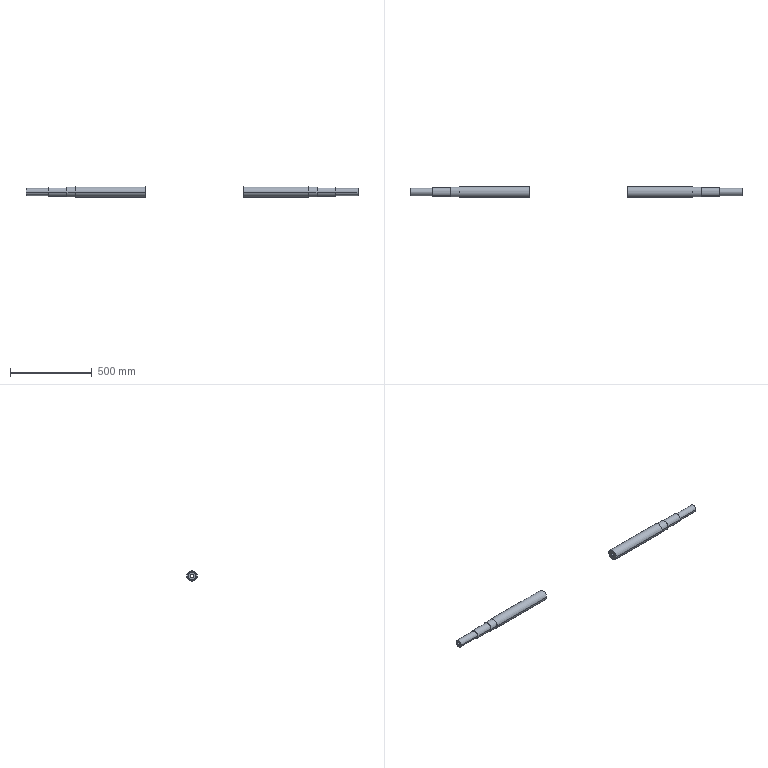Part | STEP file | Axle | 2 solids | 30 faces | box 2025 x 64 x 64 mm | volume 3440421 mm3 | cylinder 20 | plane 10 | commonest cylinder face diameters 20 x4 45 x4 54 x4 60 x4 64 x4
STEP:
#1=CARTESIAN_POINT('',(-712.5,-30.,0.));
#2=VERTEX_POINT('',#1);
#3=CARTESIAN_POINT('',(-712.5,30.,0.));
#4=VERTEX_POINT('',#3);
#5=CARTESIAN_POINT('',(-712.5,0.,0.));
#6=DIRECTION('',(-1.,0.,0.));
#7=DIRECTION('',(0.,-1.,0.));
#8=AXIS2_PLACEMENT_3D('',#5,#6,#7);
#9=CIRCLE('',#8,30.);
#10=EDGE_CURVE('',#2,#4,#9,.T.);
#11=ORIENTED_EDGE('',*,*,#10,.T.);
#12=CARTESIAN_POINT('',(-762.5,30.,0.));
#13=VERTEX_POINT('',#12);
#14=CARTESIAN_POINT('',(-1012.5,30.,0.));
#15=DIRECTION('',(-1.,0.,0.));
#16=VECTOR('',#15,1000.);
#17=LINE('',#14,#16);
#18=EDGE_CURVE('',#4,#13,#17,.T.);
#19=ORIENTED_EDGE('',*,*,#18,.T.);
#20=CARTESIAN_POINT('',(-762.5,-30.,0.));
#21=VERTEX_POINT('',#20);
#22=CARTESIAN_POINT('',(-762.5,0.,0.));
#23=DIRECTION('',(-1.,0.,0.));
#24=DIRECTION('',(0.,-1.,0.));
#25=AXIS2_PLACEMENT_3D('',#22,#23,#24);
#26=CIRCLE('',#25,30.);
#27=EDGE_CURVE('',#21,#13,#26,.T.);
#28=ORIENTED_EDGE('',*,*,#27,.F.);
#29=CARTESIAN_POINT('',(-1012.5,-30.,0.));
#30=DIRECTION('',(-1.,0.,0.));
#31=VECTOR('',#30,1000.);
#32=LINE('',#29,#31);
#33=EDGE_CURVE('',#2,#21,#32,.T.);
#34=ORIENTED_EDGE('',*,*,#33,.F.);
#35=EDGE_LOOP('',(#11,#19,#28,#34));
#36=FACE_OUTER_BOUND('',#35,.T.);
#37=CARTESIAN_POINT('',(-1012.5,0.,0.));
#38=DIRECTION('',(-1.,0.,0.));
#39=DIRECTION('',(0.,-1.,0.));
#40=AXIS2_PLACEMENT_3D('',#37,#38,#39);
#41=CYLINDRICAL_SURFACE('',#40,30.);
#42=ADVANCED_FACE('',(#36),#41,.T.);
#43=CARTESIAN_POINT('',(-762.5,-27.,0.));
#44=VERTEX_POINT('',#43);
#45=CARTESIAN_POINT('',(-762.5,27.,0.));
#46=VERTEX_POINT('',#45);
#47=CARTESIAN_POINT('',(-762.5,0.,0.));
#48=DIRECTION('',(-1.,0.,0.));
#49=DIRECTION('',(0.,-1.,0.));
#50=AXIS2_PLACEMENT_3D('',#47,#48,#49);
#51=CIRCLE('',#50,27.);
#52=EDGE_CURVE('',#44,#46,#51,.T.);
#53=ORIENTED_EDGE('',*,*,#52,.T.);
#54=CARTESIAN_POINT('',(-872.5,27.,0.));
#55=VERTEX_POINT('',#54);
#56=CARTESIAN_POINT('',(-1012.5,27.,0.));
#57=DIRECTION('',(-1.,0.,0.));
#58=VECTOR('',#57,1000.);
#59=LINE('',#56,#58);
#60=EDGE_CURVE('',#46,#55,#59,.T.);
#61=ORIENTED_EDGE('',*,*,#60,.T.);
#62=CARTESIAN_POINT('',(-872.5,-27.,0.));
#63=VERTEX_POINT('',#62);
#64=CARTESIAN_POINT('',(-872.5,0.,0.));
#65=DIRECTION('',(-1.,0.,0.));
#66=DIRECTION('',(0.,-1.,0.));
#67=AXIS2_PLACEMENT_3D('',#64,#65,#66);
#68=CIRCLE('',#67,27.);
#69=EDGE_CURVE('',#63,#55,#68,.T.);
#70=ORIENTED_EDGE('',*,*,#69,.F.);
#71=CARTESIAN_POINT('',(-1012.5,-27.,0.));
#72=DIRECTION('',(-1.,0.,0.));
#73=VECTOR('',#72,1000.);
#74=LINE('',#71,#73);
#75=EDGE_CURVE('',#44,#63,#74,.T.);
#76=ORIENTED_EDGE('',*,*,#75,.F.);
#77=EDGE_LOOP('',(#53,#61,#70,#76));
#78=FACE_OUTER_BOUND('',#77,.T.);
#79=CARTESIAN_POINT('',(-1012.5,0.,0.));
#80=DIRECTION('',(-1.,0.,0.));
#81=DIRECTION('',(0.,-1.,0.));
#82=AXIS2_PLACEMENT_3D('',#79,#80,#81);
#83=CYLINDRICAL_SURFACE('',#82,27.);
#84=ADVANCED_FACE('',(#78),#83,.T.);
#85=CARTESIAN_POINT('',(-872.5,-22.5,0.));
#86=VERTEX_POINT('',#85);
#87=CARTESIAN_POINT('',(-872.5,22.5,0.));
#88=VERTEX_POINT('',#87);
#89=CARTESIAN_POINT('',(-872.5,0.,0.));
#90=DIRECTION('',(-1.,0.,0.));
#91=DIRECTION('',(0.,-1.,0.));
#92=AXIS2_PLACEMENT_3D('',#89,#90,#91);
#93=CIRCLE('',#92,22.5);
#94=EDGE_CURVE('',#86,#88,#93,.T.);
#95=ORIENTED_EDGE('',*,*,#94,.T.);
#96=CARTESIAN_POINT('',(-1012.5,22.5,0.));
#97=VERTEX_POINT('',#96);
#98=CARTESIAN_POINT('',(-1012.5,22.5,0.));
#99=DIRECTION('',(-1.,0.,0.));
#100=VECTOR('',#99,1000.);
#101=LINE('',#98,#100);
#102=EDGE_CURVE('',#88,#97,#101,.T.);
#103=ORIENTED_EDGE('',*,*,#102,.T.);
#104=CARTESIAN_POINT('',(-1012.5,-22.5,0.));
#105=VERTEX_POINT('',#104);
#106=CARTESIAN_POINT('',(-1012.5,0.,0.));
#107=DIRECTION('',(-1.,0.,0.));
#108=DIRECTION('',(0.,-1.,0.));
#109=AXIS2_PLACEMENT_3D('',#106,#107,#108);
#110=CIRCLE('',#109,22.5);
#111=EDGE_CURVE('',#105,#97,#110,.T.);
#112=ORIENTED_EDGE('',*,*,#111,.F.);
#113=CARTESIAN_POINT('',(-1012.5,-22.5,0.));
#114=DIRECTION('',(-1.,0.,0.));
#115=VECTOR('',#114,1000.);
#116=LINE('',#113,#115);
#117=EDGE_CURVE('',#86,#105,#116,.T.);
#118=ORIENTED_EDGE('',*,*,#117,.F.);
#119=EDGE_LOOP('',(#95,#103,#112,#118));
#120=FACE_OUTER_BOUND('',#119,.T.);
#121=CARTESIAN_POINT('',(-1012.5,0.,0.));
#122=DIRECTION('',(-1.,0.,0.));
#123=DIRECTION('',(0.,-1.,0.));
#124=AXIS2_PLACEMENT_3D('',#121,#122,#123);
#125=CYLINDRICAL_SURFACE('',#124,22.5);
#126=ADVANCED_FACE('',(#120),#125,.T.);
#127=CARTESIAN_POINT('',(-284.662,-10.,0.));
#128=VERTEX_POINT('',#127);
#129=CARTESIAN_POINT('',(-284.662,10.,0.));
#130=VERTEX_POINT('',#129);
#131=CARTESIAN_POINT('',(-284.662,0.,0.));
#132=DIRECTION('',(1.,0.,0.));
#133=DIRECTION('',(0.,0.,1.));
#134=AXIS2_PLACEMENT_3D('',#131,#132,#133);
#135=CIRCLE('',#134,10.);
#136=EDGE_CURVE('',#128,#130,#135,.T.);
#137=ORIENTED_EDGE('',*,*,#136,.T.);
#138=CARTESIAN_POINT('',(-1012.5,10.,0.));
#139=VERTEX_POINT('',#138);
#140=CARTESIAN_POINT('',(1012.501,10.,0.));
#141=DIRECTION('',(-1.,0.,0.));
#142=VECTOR('',#141,1000.);
#143=LINE('',#140,#142);
#144=EDGE_CURVE('',#130,#139,#143,.T.);
#145=ORIENTED_EDGE('',*,*,#144,.T.);
#146=CARTESIAN_POINT('',(-1012.5,-10.,0.));
#147=VERTEX_POINT('',#146);
#148=CARTESIAN_POINT('',(-1012.5,0.,0.));
#149=DIRECTION('',(-1.,0.,0.));
#150=DIRECTION('',(0.,-1.,0.));
#151=AXIS2_PLACEMENT_3D('',#148,#149,#150);
#152=CIRCLE('',#151,10.);
#153=EDGE_CURVE('',#139,#147,#152,.T.);
#154=ORIENTED_EDGE('',*,*,#153,.T.);
#155=CARTESIAN_POINT('',(1012.501,-10.,0.));
#156=DIRECTION('',(-1.,0.,0.));
#157=VECTOR('',#156,1000.);
#158=LINE('',#155,#157);
#159=EDGE_CURVE('',#128,#147,#158,.T.);
#160=ORIENTED_EDGE('',*,*,#159,.F.);
#161=EDGE_LOOP('',(#137,#145,#154,#160));
#162=FACE_OUTER_BOUND('',#161,.T.);
#163=CARTESIAN_POINT('',(1012.501,0.,0.));
#164=DIRECTION('',(-1.,0.,0.));
#165=DIRECTION('',(0.,-1.,0.));
#166=AXIS2_PLACEMENT_3D('',#163,#164,#165);
#167=CYLINDRICAL_SURFACE('',#166,10.);
#168=ADVANCED_FACE('',(#162),#167,.F.);
#169=CARTESIAN_POINT('',(-284.662,-32.,0.));
#170=VERTEX_POINT('',#169);
#171=CARTESIAN_POINT('',(-284.662,32.,0.));
#172=VERTEX_POINT('',#171);
#173=CARTESIAN_POINT('',(-284.662,0.,0.));
#174=DIRECTION('',(-1.,0.,0.));
#175=DIRECTION('',(0.,0.,1.));
#176=AXIS2_PLACEMENT_3D('',#173,#174,#175);
#177=CIRCLE('',#176,32.);
#178=EDGE_CURVE('',#170,#172,#177,.T.);
#179=ORIENTED_EDGE('',*,*,#178,.T.);
#180=CARTESIAN_POINT('',(-712.5,32.,0.));
#181=VERTEX_POINT('',#180);
#182=CARTESIAN_POINT('',(-1012.5,32.,0.));
#183=DIRECTION('',(-1.,0.,0.));
#184=VECTOR('',#183,1000.);
#185=LINE('',#182,#184);
#186=EDGE_CURVE('',#172,#181,#185,.T.);
#187=ORIENTED_EDGE('',*,*,#186,.T.);
#188=CARTESIAN_POINT('',(-712.5,-32.,0.));
#189=VERTEX_POINT('',#188);
#190=CARTESIAN_POINT('',(-712.5,0.,0.));
#191=DIRECTION('',(-1.,0.,0.));
#192=DIRECTION('',(0.,-1.,0.));
#193=AXIS2_PLACEMENT_3D('',#190,#191,#192);
#194=CIRCLE('',#193,32.);
#195=EDGE_CURVE('',#189,#181,#194,.T.);
#196=ORIENTED_EDGE('',*,*,#195,.F.);
#197=CARTESIAN_POINT('',(-1012.5,-32.,0.));
#198=DIRECTION('',(-1.,0.,0.));
#199=VECTOR('',#198,1000.);
#200=LINE('',#197,#199);
#201=EDGE_CURVE('',#170,#189,#200,.T.);
#202=ORIENTED_EDGE('',*,*,#201,.F.);
#203=EDGE_LOOP('',(#179,#187,#196,#202));
#204=FACE_OUTER_BOUND('',#203,.T.);
#205=CARTESIAN_POINT('',(-1012.5,0.,0.));
#206=DIRECTION('',(-1.,0.,0.));
#207=DIRECTION('',(0.,-1.,0.));
#208=AXIS2_PLACEMENT_3D('',#205,#206,#207);
#209=CYLINDRICAL_SURFACE('',#208,32.);
#210=ADVANCED_FACE('',(#204),#209,.T.);
#211=ORIENTED_EDGE('',*,*,#186,.F.);
#212=CARTESIAN_POINT('',(-284.662,0.,0.));
#213=DIRECTION('',(-1.,0.,0.));
#214=DIRECTION('',(0.,0.,1.));
#215=AXIS2_PLACEMENT_3D('',#212,#213,#214);
#216=CIRCLE('',#215,32.);
#217=EDGE_CURVE('',#172,#170,#216,.T.);
#218=ORIENTED_EDGE('',*,*,#217,.T.);
#219=ORIENTED_EDGE('',*,*,#201,.T.);
#220=CARTESIAN_POINT('',(-712.5,0.,0.));
#221=DIRECTION('',(-1.,0.,0.));
#222=DIRECTION('',(0.,-1.,0.));
#223=AXIS2_PLACEMENT_3D('',#220,#221,#222);
#224=CIRCLE('',#223,32.);
#225=EDGE_CURVE('',#181,#189,#224,.T.);
#226=ORIENTED_EDGE('',*,*,#225,.F.);
#227=EDGE_LOOP('',(#211,#218,#219,#226));
#228=FACE_OUTER_BOUND('',#227,.T.);
#229=CARTESIAN_POINT('',(-1012.5,0.,0.));
#230=DIRECTION('',(-1.,0.,0.));
#231=DIRECTION('',(0.,-1.,0.));
#232=AXIS2_PLACEMENT_3D('',#229,#230,#231);
#233=CYLINDRICAL_SURFACE('',#232,32.);
#234=ADVANCED_FACE('',(#228),#233,.T.);
#235=ORIENTED_EDGE('',*,*,#144,.F.);
#236=CARTESIAN_POINT('',(-284.662,0.,0.));
#237=DIRECTION('',(1.,0.,0.));
#238=DIRECTION('',(0.,0.,1.));
#239=AXIS2_PLACEMENT_3D('',#236,#237,#238);
#240=CIRCLE('',#239,10.);
#241=EDGE_CURVE('',#130,#128,#240,.T.);
#242=ORIENTED_EDGE('',*,*,#241,.T.);
#243=ORIENTED_EDGE('',*,*,#159,.T.);
#244=CARTESIAN_POINT('',(-1012.5,0.,0.));
#245=DIRECTION('',(-1.,0.,0.));
#246=DIRECTION('',(0.,-1.,0.));
#247=AXIS2_PLACEMENT_3D('',#244,#245,#246);
#248=CIRCLE('',#247,10.);
#249=EDGE_CURVE('',#147,#139,#248,.T.);
#250=ORIENTED_EDGE('',*,*,#249,.T.);
#251=EDGE_LOOP('',(#235,#242,#243,#250));
#252=FACE_OUTER_BOUND('',#251,.T.);
#253=CARTESIAN_POINT('',(1012.501,0.,0.));
#254=DIRECTION('',(-1.,0.,0.));
#255=DIRECTION('',(0.,-1.,0.));
#256=AXIS2_PLACEMENT_3D('',#253,#254,#255);
#257=CYLINDRICAL_SURFACE('',#256,10.);
#258=ADVANCED_FACE('',(#252),#257,.F.);
#259=ORIENTED_EDGE('',*,*,#249,.F.);
#260=ORIENTED_EDGE('',*,*,#153,.F.);
#261=EDGE_LOOP('',(#259,#260));
#262=FACE_BOUND('',#261,.T.);
#263=ORIENTED_EDGE('',*,*,#111,.T.);
#264=CARTESIAN_POINT('',(-1012.5,0.,0.));
#265=DIRECTION('',(-1.,0.,0.));
#266=DIRECTION('',(0.,-1.,0.));
#267=AXIS2_PLACEMENT_3D('',#264,#265,#266);
#268=CIRCLE('',#267,22.5);
#269=EDGE_CURVE('',#97,#105,#268,.T.);
#270=ORIENTED_EDGE('',*,*,#269,.T.);
#271=EDGE_LOOP('',(#263,#270));
#272=FACE_OUTER_BOUND('',#271,.T.);
#273=CARTESIAN_POINT('',(-1012.5,0.,0.));
#274=DIRECTION('',(1.,0.,0.));
#275=DIRECTION('',(0.,1.,0.));
#276=AXIS2_PLACEMENT_3D('',#273,#274,#275);
#277=PLANE('',#276);
#278=ADVANCED_FACE('',(#262,#272),#277,.F.);
#279=ORIENTED_EDGE('',*,*,#102,.F.);
#280=CARTESIAN_POINT('',(-872.5,0.,0.));
#281=DIRECTION('',(-1.,0.,0.));
#282=DIRECTION('',(0.,-1.,0.));
#283=AXIS2_PLACEMENT_3D('',#280,#281,#282);
#284=CIRCLE('',#283,22.5);
#285=EDGE_CURVE('',#88,#86,#284,.T.);
#286=ORIENTED_EDGE('',*,*,#285,.T.);
#287=ORIENTED_EDGE('',*,*,#117,.T.);
#288=ORIENTED_EDGE('',*,*,#269,.F.);
#289=EDGE_LOOP('',(#279,#286,#287,#288));
#290=FACE_OUTER_BOUND('',#289,.T.);
#291=CARTESIAN_POINT('',(-1012.5,0.,0.));
#292=DIRECTION('',(-1.,0.,0.));
#293=DIRECTION('',(0.,-1.,0.));
#294=AXIS2_PLACEMENT_3D('',#291,#292,#293);
#295=CYLINDRICAL_SURFACE('',#294,22.5);
#296=ADVANCED_FACE('',(#290),#295,.T.);
#297=ORIENTED_EDGE('',*,*,#94,.F.);
#298=ORIENTED_EDGE('',*,*,#285,.F.);
#299=EDGE_LOOP('',(#297,#298));
#300=FACE_BOUND('',#299,.T.);
#301=ORIENTED_EDGE('',*,*,#69,.T.);
#302=CARTESIAN_POINT('',(-872.5,0.,0.));
#303=DIRECTION('',(-1.,0.,0.));
#304=DIRECTION('',(0.,-1.,0.));
#305=AXIS2_PLACEMENT_3D('',#302,#303,#304);
#306=CIRCLE('',#305,27.);
#307=EDGE_CURVE('',#55,#63,#306,.T.);
#308=ORIENTED_EDGE('',*,*,#307,.T.);
#309=EDGE_LOOP('',(#301,#308));
#310=FACE_OUTER_BOUND('',#309,.T.);
#311=CARTESIAN_POINT('',(-872.5,22.5,0.));
#312=DIRECTION('',(1.,0.,0.));
#313=DIRECTION('',(0.,1.,0.));
#314=AXIS2_PLACEMENT_3D('',#311,#312,#313);
#315=PLANE('',#314);
#316=ADVANCED_FACE('',(#300,#310),#315,.F.);
#317=ORIENTED_EDGE('',*,*,#60,.F.);
#318=CARTESIAN_POINT('',(-762.5,0.,0.));
#319=DIRECTION('',(-1.,0.,0.));
#320=DIRECTION('',(0.,-1.,0.));
#321=AXIS2_PLACEMENT_3D('',#318,#319,#320);
#322=CIRCLE('',#321,27.);
#323=EDGE_CURVE('',#46,#44,#322,.T.);
#324=ORIENTED_EDGE('',*,*,#323,.T.);
#325=ORIENTED_EDGE('',*,*,#75,.T.);
#326=ORIENTED_EDGE('',*,*,#307,.F.);
#327=EDGE_LOOP('',(#317,#324,#325,#326));
#328=FACE_OUTER_BOUND('',#327,.T.);
#329=CARTESIAN_POINT('',(-1012.5,0.,0.));
#330=DIRECTION('',(-1.,0.,0.));
#331=DIRECTION('',(0.,-1.,0.));
#332=AXIS2_PLACEMENT_3D('',#329,#330,#331);
#333=CYLINDRICAL_SURFACE('',#332,27.);
#334=ADVANCED_FACE('',(#328),#333,.T.);
#335=ORIENTED_EDGE('',*,*,#52,.F.);
#336=ORIENTED_EDGE('',*,*,#323,.F.);
#337=EDGE_LOOP('',(#335,#336));
#338=FACE_BOUND('',#337,.T.);
#339=ORIENTED_EDGE('',*,*,#27,.T.);
#340=CARTESIAN_POINT('',(-762.5,0.,0.));
#341=DIRECTION('',(-1.,0.,0.));
#342=DIRECTION('',(0.,-1.,0.));
#343=AXIS2_PLACEMENT_3D('',#340,#341,#342);
#344=CIRCLE('',#343,30.);
#345=EDGE_CURVE('',#13,#21,#344,.T.);
#346=ORIENTED_EDGE('',*,*,#345,.T.);
#347=EDGE_LOOP('',(#339,#346));
#348=FACE_OUTER_BOUND('',#347,.T.);
#349=CARTESIAN_POINT('',(-762.5,30.,0.));
#350=DIRECTION('',(1.,0.,0.));
#351=DIRECTION('',(0.,1.,0.));
#352=AXIS2_PLACEMENT_3D('',#349,#350,#351);
#353=PLANE('',#352);
#354=ADVANCED_FACE('',(#338,#348),#353,.F.);
#355=ORIENTED_EDGE('',*,*,#18,.F.);
#356=CARTESIAN_POINT('',(-712.5,0.,0.));
#357=DIRECTION('',(-1.,0.,0.));
#358=DIRECTION('',(0.,-1.,0.));
#359=AXIS2_PLACEMENT_3D('',#356,#357,#358);
#360=CIRCLE('',#359,30.);
#361=EDGE_CURVE('',#4,#2,#360,.T.);
#362=ORIENTED_EDGE('',*,*,#361,.T.);
#363=ORIENTED_EDGE('',*,*,#33,.T.);
#364=ORIENTED_EDGE('',*,*,#345,.F.);
#365=EDGE_LOOP('',(#355,#362,#363,#364));
#366=FACE_OUTER_BOUND('',#365,.T.);
#367=CARTESIAN_POINT('',(-1012.5,0.,0.));
#368=DIRECTION('',(-1.,0.,0.));
#369=DIRECTION('',(0.,-1.,0.));
#370=AXIS2_PLACEMENT_3D('',#367,#368,#369);
#371=CYLINDRICAL_SURFACE('',#370,30.);
#372=ADVANCED_FACE('',(#366),#371,.T.);
#373=ORIENTED_EDGE('',*,*,#10,.F.);
#374=ORIENTED_EDGE('',*,*,#361,.F.);
#375=EDGE_LOOP('',(#373,#374));
#376=FACE_BOUND('',#375,.T.);
#377=ORIENTED_EDGE('',*,*,#195,.T.);
#378=ORIENTED_EDGE('',*,*,#225,.T.);
#379=EDGE_LOOP('',(#377,#378));
#380=FACE_OUTER_BOUND('',#379,.T.);
#381=CARTESIAN_POINT('',(-712.5,30.,0.));
#382=DIRECTION('',(1.,0.,0.));
#383=DIRECTION('',(0.,1.,0.));
#384=AXIS2_PLACEMENT_3D('',#381,#382,#383);
#385=PLANE('',#384);
#386=ADVANCED_FACE('',(#376,#380),#385,.F.);
#387=ORIENTED_EDGE('',*,*,#136,.F.);
#388=ORIENTED_EDGE('',*,*,#241,.F.);
#389=EDGE_LOOP('',(#387,#388));
#390=FACE_BOUND('',#389,.T.);
#391=ORIENTED_EDGE('',*,*,#178,.F.);
#392=ORIENTED_EDGE('',*,*,#217,.F.);
#393=EDGE_LOOP('',(#391,#392));
#394=FACE_OUTER_BOUND('',#393,.T.);
#395=CARTESIAN_POINT('',(-284.662,-103.,59.586));
#396=DIRECTION('',(-1.,0.,0.));
#397=DIRECTION('',(0.,0.,1.));
#398=AXIS2_PLACEMENT_3D('',#395,#396,#397);
#399=PLANE('',#398);
#400=ADVANCED_FACE('',(#390,#394),#399,.F.);
#401=CLOSED_SHELL('',(#42,#84,#126,#168,#210,#234,#258,#278,#296,#316,#334,#354,#372,#386,#400));
#402=MANIFOLD_SOLID_BREP('',#401);
#403=CARTESIAN_POINT('',(1012.5,-10.,0.));
#404=VERTEX_POINT('',#403);
#405=CARTESIAN_POINT('',(1012.5,10.,0.));
#406=VERTEX_POINT('',#405);
#407=CARTESIAN_POINT('',(1012.5,0.,0.));
#408=DIRECTION('',(1.,0.,0.));
#409=DIRECTION('',(0.,-1.,0.));
#410=AXIS2_PLACEMENT_3D('',#407,#408,#409);
#411=CIRCLE('',#410,10.);
#412=EDGE_CURVE('',#404,#406,#411,.T.);
#413=ORIENTED_EDGE('',*,*,#412,.T.);
#414=CARTESIAN_POINT('',(314.592,10.,0.));
#415=VERTEX_POINT('',#414);
#416=CARTESIAN_POINT('',(1012.501,10.,0.));
#417=DIRECTION('',(-1.,0.,0.));
#418=VECTOR('',#417,1000.);
#419=LINE('',#416,#418);
#420=EDGE_CURVE('',#406,#415,#419,.T.);
#421=ORIENTED_EDGE('',*,*,#420,.T.);
#422=CARTESIAN_POINT('',(314.592,-10.,0.));
#423=VERTEX_POINT('',#422);
#424=CARTESIAN_POINT('',(314.592,0.,0.));
#425=DIRECTION('',(-1.,0.,0.));
#426=DIRECTION('',(0.,0.,-1.));
#427=AXIS2_PLACEMENT_3D('',#424,#425,#426);
#428=CIRCLE('',#427,10.);
#429=EDGE_CURVE('',#415,#423,#428,.T.);
#430=ORIENTED_EDGE('',*,*,#429,.T.);
#431=CARTESIAN_POINT('',(1012.501,-10.,0.));
#432=DIRECTION('',(-1.,0.,0.));
#433=VECTOR('',#432,1000.);
#434=LINE('',#431,#433);
#435=EDGE_CURVE('',#404,#423,#434,.T.);
#436=ORIENTED_EDGE('',*,*,#435,.F.);
#437=EDGE_LOOP('',(#413,#421,#430,#436));
#438=FACE_OUTER_BOUND('',#437,.T.);
#439=CARTESIAN_POINT('',(1012.501,0.,0.));
#440=DIRECTION('',(-1.,0.,0.));
#441=DIRECTION('',(0.,-1.,0.));
#442=AXIS2_PLACEMENT_3D('',#439,#440,#441);
#443=CYLINDRICAL_SURFACE('',#442,10.);
#444=ADVANCED_FACE('',(#438),#443,.F.);
#445=CARTESIAN_POINT('',(1012.5,-22.5,0.));
#446=VERTEX_POINT('',#445);
#447=CARTESIAN_POINT('',(1012.5,22.5,0.));
#448=VERTEX_POINT('',#447);
#449=CARTESIAN_POINT('',(1012.5,0.,0.));
#450=DIRECTION('',(-1.,0.,0.));
#451=DIRECTION('',(0.,-1.,0.));
#452=AXIS2_PLACEMENT_3D('',#449,#450,#451);
#453=CIRCLE('',#452,22.5);
#454=EDGE_CURVE('',#446,#448,#453,.T.);
#455=ORIENTED_EDGE('',*,*,#454,.T.);
#456=CARTESIAN_POINT('',(872.5,22.5,0.));
#457=VERTEX_POINT('',#456);
#458=CARTESIAN_POINT('',(-1012.5,22.5,0.));
#459=DIRECTION('',(-1.,0.,0.));
#460=VECTOR('',#459,1000.);
#461=LINE('',#458,#460);
#462=EDGE_CURVE('',#448,#457,#461,.T.);
#463=ORIENTED_EDGE('',*,*,#462,.T.);
#464=CARTESIAN_POINT('',(872.5,-22.5,0.));
#465=VERTEX_POINT('',#464);
#466=CARTESIAN_POINT('',(872.5,0.,0.));
#467=DIRECTION('',(-1.,0.,0.));
#468=DIRECTION('',(0.,-1.,0.));
#469=AXIS2_PLACEMENT_3D('',#466,#467,#468);
#470=CIRCLE('',#469,22.5);
#471=EDGE_CURVE('',#465,#457,#470,.T.);
#472=ORIENTED_EDGE('',*,*,#471,.F.);
#473=CARTESIAN_POINT('',(-1012.5,-22.5,0.));
#474=DIRECTION('',(-1.,0.,0.));
#475=VECTOR('',#474,1000.);
#476=LINE('',#473,#475);
#477=EDGE_CURVE('',#446,#465,#476,.T.);
#478=ORIENTED_EDGE('',*,*,#477,.F.);
#479=EDGE_LOOP('',(#455,#463,#472,#478));
#480=FACE_OUTER_BOUND('',#479,.T.);
#481=CARTESIAN_POINT('',(-1012.5,0.,0.));
#482=DIRECTION('',(-1.,0.,0.));
#483=DIRECTION('',(0.,-1.,0.));
#484=AXIS2_PLACEMENT_3D('',#481,#482,#483);
#485=CYLINDRICAL_SURFACE('',#484,22.5);
#486=ADVANCED_FACE('',(#480),#485,.T.);
#487=CARTESIAN_POINT('',(872.5,-27.,0.));
#488=VERTEX_POINT('',#487);
#489=CARTESIAN_POINT('',(872.5,27.,0.));
#490=VERTEX_POINT('',#489);
#491=CARTESIAN_POINT('',(872.5,0.,0.));
#492=DIRECTION('',(-1.,0.,0.));
#493=DIRECTION('',(0.,-1.,0.));
#494=AXIS2_PLACEMENT_3D('',#491,#492,#493);
#495=CIRCLE('',#494,27.);
#496=EDGE_CURVE('',#488,#490,#495,.T.);
#497=ORIENTED_EDGE('',*,*,#496,.T.);
#498=CARTESIAN_POINT('',(762.5,27.,0.));
#499=VERTEX_POINT('',#498);
#500=CARTESIAN_POINT('',(-1012.5,27.,0.));
#501=DIRECTION('',(-1.,0.,0.));
#502=VECTOR('',#501,1000.);
#503=LINE('',#500,#502);
#504=EDGE_CURVE('',#490,#499,#503,.T.);
#505=ORIENTED_EDGE('',*,*,#504,.T.);
#506=CARTESIAN_POINT('',(762.5,-27.,0.));
#507=VERTEX_POINT('',#506);
#508=CARTESIAN_POINT('',(762.5,0.,0.));
#509=DIRECTION('',(-1.,0.,0.));
#510=DIRECTION('',(0.,-1.,0.));
#511=AXIS2_PLACEMENT_3D('',#508,#509,#510);
#512=CIRCLE('',#511,27.);
#513=EDGE_CURVE('',#507,#499,#512,.T.);
#514=ORIENTED_EDGE('',*,*,#513,.F.);
#515=CARTESIAN_POINT('',(-1012.5,-27.,0.));
#516=DIRECTION('',(-1.,0.,0.));
#517=VECTOR('',#516,1000.);
#518=LINE('',#515,#517);
#519=EDGE_CURVE('',#488,#507,#518,.T.);
#520=ORIENTED_EDGE('',*,*,#519,.F.);
#521=EDGE_LOOP('',(#497,#505,#514,#520));
#522=FACE_OUTER_BOUND('',#521,.T.);
#523=CARTESIAN_POINT('',(-1012.5,0.,0.));
#524=DIRECTION('',(-1.,0.,0.));
#525=DIRECTION('',(0.,-1.,0.));
#526=AXIS2_PLACEMENT_3D('',#523,#524,#525);
#527=CYLINDRICAL_SURFACE('',#526,27.);
#528=ADVANCED_FACE('',(#522),#527,.T.);
#529=CARTESIAN_POINT('',(712.5,-32.,0.));
#530=VERTEX_POINT('',#529);
#531=CARTESIAN_POINT('',(712.5,32.,0.));
#532=VERTEX_POINT('',#531);
#533=CARTESIAN_POINT('',(712.5,0.,0.));
#534=DIRECTION('',(-1.,0.,0.));
#535=DIRECTION('',(0.,-1.,0.));
#536=AXIS2_PLACEMENT_3D('',#533,#534,#535);
#537=CIRCLE('',#536,32.);
#538=EDGE_CURVE('',#530,#532,#537,.T.);
#539=ORIENTED_EDGE('',*,*,#538,.T.);
#540=CARTESIAN_POINT('',(314.592,32.,0.));
#541=VERTEX_POINT('',#540);
#542=CARTESIAN_POINT('',(-1012.5,32.,0.));
#543=DIRECTION('',(-1.,0.,0.));
#544=VECTOR('',#543,1000.);
#545=LINE('',#542,#544);
#546=EDGE_CURVE('',#532,#541,#545,.T.);
#547=ORIENTED_EDGE('',*,*,#546,.T.);
#548=CARTESIAN_POINT('',(314.592,-32.,0.));
#549=VERTEX_POINT('',#548);
#550=CARTESIAN_POINT('',(314.592,0.,0.));
#551=DIRECTION('',(1.,0.,0.));
#552=DIRECTION('',(0.,0.,-1.));
#553=AXIS2_PLACEMENT_3D('',#550,#551,#552);
#554=CIRCLE('',#553,32.);
#555=EDGE_CURVE('',#541,#549,#554,.T.);
#556=ORIENTED_EDGE('',*,*,#555,.T.);
#557=CARTESIAN_POINT('',(-1012.5,-32.,0.));
#558=DIRECTION('',(-1.,0.,0.));
#559=VECTOR('',#558,1000.);
#560=LINE('',#557,#559);
#561=EDGE_CURVE('',#530,#549,#560,.T.);
#562=ORIENTED_EDGE('',*,*,#561,.F.);
#563=EDGE_LOOP('',(#539,#547,#556,#562));
#564=FACE_OUTER_BOUND('',#563,.T.);
#565=CARTESIAN_POINT('',(-1012.5,0.,0.));
#566=DIRECTION('',(-1.,0.,0.));
#567=DIRECTION('',(0.,-1.,0.));
#568=AXIS2_PLACEMENT_3D('',#565,#566,#567);
#569=CYLINDRICAL_SURFACE('',#568,32.);
#570=ADVANCED_FACE('',(#564),#569,.T.);
#571=CARTESIAN_POINT('',(762.5,-30.,0.));
#572=VERTEX_POINT('',#571);
#573=CARTESIAN_POINT('',(762.5,30.,0.));
#574=VERTEX_POINT('',#573);
#575=CARTESIAN_POINT('',(762.5,0.,0.));
#576=DIRECTION('',(-1.,0.,0.));
#577=DIRECTION('',(0.,-1.,0.));
#578=AXIS2_PLACEMENT_3D('',#575,#576,#577);
#579=CIRCLE('',#578,30.);
#580=EDGE_CURVE('',#572,#574,#579,.T.);
#581=ORIENTED_EDGE('',*,*,#580,.T.);
#582=CARTESIAN_POINT('',(712.5,30.,0.));
#583=VERTEX_POINT('',#582);
#584=CARTESIAN_POINT('',(-1012.5,30.,0.));
#585=DIRECTION('',(-1.,0.,0.));
#586=VECTOR('',#585,1000.);
#587=LINE('',#584,#586);
#588=EDGE_CURVE('',#574,#583,#587,.T.);
#589=ORIENTED_EDGE('',*,*,#588,.T.);
#590=CARTESIAN_POINT('',(712.5,-30.,0.));
#591=VERTEX_POINT('',#590);
#592=CARTESIAN_POINT('',(712.5,0.,0.));
#593=DIRECTION('',(-1.,0.,0.));
#594=DIRECTION('',(0.,-1.,0.));
#595=AXIS2_PLACEMENT_3D('',#592,#593,#594);
#596=CIRCLE('',#595,30.);
#597=EDGE_CURVE('',#591,#583,#596,.T.);
#598=ORIENTED_EDGE('',*,*,#597,.F.);
#599=CARTESIAN_POINT('',(-1012.5,-30.,0.));
#600=DIRECTION('',(-1.,0.,0.));
#601=VECTOR('',#600,1000.);
#602=LINE('',#599,#601);
#603=EDGE_CURVE('',#572,#591,#602,.T.);
#604=ORIENTED_EDGE('',*,*,#603,.F.);
#605=EDGE_LOOP('',(#581,#589,#598,#604));
#606=FACE_OUTER_BOUND('',#605,.T.);
#607=CARTESIAN_POINT('',(-1012.5,0.,0.));
#608=DIRECTION('',(-1.,0.,0.));
#609=DIRECTION('',(0.,-1.,0.));
#610=AXIS2_PLACEMENT_3D('',#607,#608,#609);
#611=CYLINDRICAL_SURFACE('',#610,30.);
#612=ADVANCED_FACE('',(#606),#611,.T.);
#613=ORIENTED_EDGE('',*,*,#580,.F.);
#614=CARTESIAN_POINT('',(762.5,0.,0.));
#615=DIRECTION('',(-1.,0.,0.));
#616=DIRECTION('',(0.,-1.,0.));
#617=AXIS2_PLACEMENT_3D('',#614,#615,#616);
#618=CIRCLE('',#617,30.);
#619=EDGE_CURVE('',#574,#572,#618,.T.);
#620=ORIENTED_EDGE('',*,*,#619,.F.);
#621=EDGE_LOOP('',(#613,#620));
#622=FACE_OUTER_BOUND('',#621,.T.);
#623=ORIENTED_EDGE('',*,*,#513,.T.);
#624=CARTESIAN_POINT('',(762.5,0.,0.));
#625=DIRECTION('',(-1.,0.,0.));
#626=DIRECTION('',(0.,-1.,0.));
#627=AXIS2_PLACEMENT_3D('',#624,#625,#626);
#628=CIRCLE('',#627,27.);
#629=EDGE_CURVE('',#499,#507,#628,.T.);
#630=ORIENTED_EDGE('',*,*,#629,.T.);
#631=EDGE_LOOP('',(#623,#630));
#632=FACE_BOUND('',#631,.T.);
#633=CARTESIAN_POINT('',(762.5,30.,0.));
#634=DIRECTION('',(-1.,0.,0.));
#635=DIRECTION('',(0.,-1.,0.));
#636=AXIS2_PLACEMENT_3D('',#633,#634,#635);
#637=PLANE('',#636);
#638=ADVANCED_FACE('',(#622,#632),#637,.F.);
#639=ORIENTED_EDGE('',*,*,#588,.F.);
#640=ORIENTED_EDGE('',*,*,#619,.T.);
#641=ORIENTED_EDGE('',*,*,#603,.T.);
#642=CARTESIAN_POINT('',(712.5,0.,0.));
#643=DIRECTION('',(-1.,0.,0.));
#644=DIRECTION('',(0.,-1.,0.));
#645=AXIS2_PLACEMENT_3D('',#642,#643,#644);
#646=CIRCLE('',#645,30.);
#647=EDGE_CURVE('',#583,#591,#646,.T.);
#648=ORIENTED_EDGE('',*,*,#647,.F.);
#649=EDGE_LOOP('',(#639,#640,#641,#648));
#650=FACE_OUTER_BOUND('',#649,.T.);
#651=CARTESIAN_POINT('',(-1012.5,0.,0.));
#652=DIRECTION('',(-1.,0.,0.));
#653=DIRECTION('',(0.,-1.,0.));
#654=AXIS2_PLACEMENT_3D('',#651,#652,#653);
#655=CYLINDRICAL_SURFACE('',#654,30.);
#656=ADVANCED_FACE('',(#650),#655,.T.);
#657=ORIENTED_EDGE('',*,*,#538,.F.);
#658=CARTESIAN_POINT('',(712.5,0.,0.));
#659=DIRECTION('',(-1.,0.,0.));
#660=DIRECTION('',(0.,-1.,0.));
#661=AXIS2_PLACEMENT_3D('',#658,#659,#660);
#662=CIRCLE('',#661,32.);
#663=EDGE_CURVE('',#532,#530,#662,.T.);
#664=ORIENTED_EDGE('',*,*,#663,.F.);
#665=EDGE_LOOP('',(#657,#664));
#666=FACE_OUTER_BOUND('',#665,.T.);
#667=ORIENTED_EDGE('',*,*,#597,.T.);
#668=ORIENTED_EDGE('',*,*,#647,.T.);
#669=EDGE_LOOP('',(#667,#668));
#670=FACE_BOUND('',#669,.T.);
#671=CARTESIAN_POINT('',(712.5,30.,0.));
#672=DIRECTION('',(-1.,0.,0.));
#673=DIRECTION('',(0.,-1.,0.));
#674=AXIS2_PLACEMENT_3D('',#671,#672,#673);
#675=PLANE('',#674);
#676=ADVANCED_FACE('',(#666,#670),#675,.F.);
#677=ORIENTED_EDGE('',*,*,#546,.F.);
#678=ORIENTED_EDGE('',*,*,#663,.T.);
#679=ORIENTED_EDGE('',*,*,#561,.T.);
#680=CARTESIAN_POINT('',(314.592,0.,0.));
#681=DIRECTION('',(1.,0.,0.));
#682=DIRECTION('',(0.,0.,-1.));
#683=AXIS2_PLACEMENT_3D('',#680,#681,#682);
#684=CIRCLE('',#683,32.);
#685=EDGE_CURVE('',#549,#541,#684,.T.);
#686=ORIENTED_EDGE('',*,*,#685,.T.);
#687=EDGE_LOOP('',(#677,#678,#679,#686));
#688=FACE_OUTER_BOUND('',#687,.T.);
#689=CARTESIAN_POINT('',(-1012.5,0.,0.));
#690=DIRECTION('',(-1.,0.,0.));
#691=DIRECTION('',(0.,-1.,0.));
#692=AXIS2_PLACEMENT_3D('',#689,#690,#691);
#693=CYLINDRICAL_SURFACE('',#692,32.);
#694=ADVANCED_FACE('',(#688),#693,.T.);
#695=ORIENTED_EDGE('',*,*,#504,.F.);
#696=CARTESIAN_POINT('',(872.5,0.,0.));
#697=DIRECTION('',(-1.,0.,0.));
#698=DIRECTION('',(0.,-1.,0.));
#699=AXIS2_PLACEMENT_3D('',#696,#697,#698);
#700=CIRCLE('',#699,27.);
#701=EDGE_CURVE('',#490,#488,#700,.T.);
#702=ORIENTED_EDGE('',*,*,#701,.T.);
#703=ORIENTED_EDGE('',*,*,#519,.T.);
#704=ORIENTED_EDGE('',*,*,#629,.F.);
#705=EDGE_LOOP('',(#695,#702,#703,#704));
#706=FACE_OUTER_BOUND('',#705,.T.);
#707=CARTESIAN_POINT('',(-1012.5,0.,0.));
#708=DIRECTION('',(-1.,0.,0.));
#709=DIRECTION('',(0.,-1.,0.));
#710=AXIS2_PLACEMENT_3D('',#707,#708,#709);
#711=CYLINDRICAL_SURFACE('',#710,27.);
#712=ADVANCED_FACE('',(#706),#711,.T.);
#713=ORIENTED_EDGE('',*,*,#496,.F.);
#714=ORIENTED_EDGE('',*,*,#701,.F.);
#715=EDGE_LOOP('',(#713,#714));
#716=FACE_OUTER_BOUND('',#715,.T.);
#717=ORIENTED_EDGE('',*,*,#471,.T.);
#718=CARTESIAN_POINT('',(872.5,0.,0.));
#719=DIRECTION('',(-1.,0.,0.));
#720=DIRECTION('',(0.,-1.,0.));
#721=AXIS2_PLACEMENT_3D('',#718,#719,#720);
#722=CIRCLE('',#721,22.5);
#723=EDGE_CURVE('',#457,#465,#722,.T.);
#724=ORIENTED_EDGE('',*,*,#723,.T.);
#725=EDGE_LOOP('',(#717,#724));
#726=FACE_BOUND('',#725,.T.);
#727=CARTESIAN_POINT('',(872.5,22.5,0.));
#728=DIRECTION('',(-1.,0.,0.));
#729=DIRECTION('',(0.,-1.,0.));
#730=AXIS2_PLACEMENT_3D('',#727,#728,#729);
#731=PLANE('',#730);
#732=ADVANCED_FACE('',(#716,#726),#731,.F.);
#733=ORIENTED_EDGE('',*,*,#462,.F.);
#734=CARTESIAN_POINT('',(1012.5,0.,0.));
#735=DIRECTION('',(-1.,0.,0.));
#736=DIRECTION('',(0.,-1.,0.));
#737=AXIS2_PLACEMENT_3D('',#734,#735,#736);
#738=CIRCLE('',#737,22.5);
#739=EDGE_CURVE('',#448,#446,#738,.T.);
#740=ORIENTED_EDGE('',*,*,#739,.T.);
#741=ORIENTED_EDGE('',*,*,#477,.T.);
#742=ORIENTED_EDGE('',*,*,#723,.F.);
#743=EDGE_LOOP('',(#733,#740,#741,#742));
#744=FACE_OUTER_BOUND('',#743,.T.);
#745=CARTESIAN_POINT('',(-1012.5,0.,0.));
#746=DIRECTION('',(-1.,0.,0.));
#747=DIRECTION('',(0.,-1.,0.));
#748=AXIS2_PLACEMENT_3D('',#745,#746,#747);
#749=CYLINDRICAL_SURFACE('',#748,22.5);
#750=ADVANCED_FACE('',(#744),#749,.T.);
#751=ORIENTED_EDGE('',*,*,#412,.F.);
#752=CARTESIAN_POINT('',(1012.5,0.,0.));
#753=DIRECTION('',(1.,0.,0.));
#754=DIRECTION('',(0.,-1.,0.));
#755=AXIS2_PLACEMENT_3D('',#752,#753,#754);
#756=CIRCLE('',#755,10.);
#757=EDGE_CURVE('',#406,#404,#756,.T.);
#758=ORIENTED_EDGE('',*,*,#757,.F.);
#759=EDGE_LOOP('',(#751,#758));
#760=FACE_BOUND('',#759,.T.);
#761=ORIENTED_EDGE('',*,*,#454,.F.);
#762=ORIENTED_EDGE('',*,*,#739,.F.);
#763=EDGE_LOOP('',(#761,#762));
#764=FACE_OUTER_BOUND('',#763,.T.);
#765=CARTESIAN_POINT('',(1012.5,0.,0.));
#766=DIRECTION('',(-1.,0.,0.));
#767=DIRECTION('',(0.,-1.,0.));
#768=AXIS2_PLACEMENT_3D('',#765,#766,#767);
#769=PLANE('',#768);
#770=ADVANCED_FACE('',(#760,#764),#769,.F.);
#771=ORIENTED_EDGE('',*,*,#420,.F.);
#772=ORIENTED_EDGE('',*,*,#757,.T.);
#773=ORIENTED_EDGE('',*,*,#435,.T.);
#774=CARTESIAN_POINT('',(314.592,0.,0.));
#775=DIRECTION('',(-1.,0.,0.));
#776=DIRECTION('',(0.,0.,-1.));
#777=AXIS2_PLACEMENT_3D('',#774,#775,#776);
#778=CIRCLE('',#777,10.);
#779=EDGE_CURVE('',#423,#415,#778,.T.);
#780=ORIENTED_EDGE('',*,*,#779,.T.);
#781=EDGE_LOOP('',(#771,#772,#773,#780));
#782=FACE_OUTER_BOUND('',#781,.T.);
#783=CARTESIAN_POINT('',(1012.501,0.,0.));
#784=DIRECTION('',(-1.,0.,0.));
#785=DIRECTION('',(0.,-1.,0.));
#786=AXIS2_PLACEMENT_3D('',#783,#784,#785);
#787=CYLINDRICAL_SURFACE('',#786,10.);
#788=ADVANCED_FACE('',(#782),#787,.F.);
#789=ORIENTED_EDGE('',*,*,#779,.F.);
#790=ORIENTED_EDGE('',*,*,#429,.F.);
#791=EDGE_LOOP('',(#789,#790));
#792=FACE_BOUND('',#791,.T.);
#793=ORIENTED_EDGE('',*,*,#685,.F.);
#794=ORIENTED_EDGE('',*,*,#555,.F.);
#795=EDGE_LOOP('',(#793,#794));
#796=FACE_OUTER_BOUND('',#795,.T.);
#797=CARTESIAN_POINT('',(314.592,-103.,59.586));
#798=DIRECTION('',(1.,0.,0.));
#799=DIRECTION('',(0.,0.,-1.));
#800=AXIS2_PLACEMENT_3D('',#797,#798,#799);
#801=PLANE('',#800);
#802=ADVANCED_FACE('',(#792,#796),#801,.F.);
#803=CLOSED_SHELL('',(#444,#486,#528,#570,#612,#638,#656,#676,#694,#712,#732,#750,#770,#788,#802));
#804=MANIFOLD_SOLID_BREP('',#803);
#805=CARTESIAN_POINT('',(0.,0.,0.));
#806=DIRECTION('',(0.,0.,1.));
#807=DIRECTION('',(1.,0.,0.));
#808=AXIS2_PLACEMENT_3D('',#805,#806,#807);
#809=(LENGTH_UNIT()NAMED_UNIT(*)SI_UNIT(.MILLI.,.METRE.));
#810=UNCERTAINTY_MEASURE_WITH_UNIT(LENGTH_MEASURE(0.00001),#809,'','');
#811=(NAMED_UNIT(*)PLANE_ANGLE_UNIT()SI_UNIT($,.RADIAN.));
#812=(NAMED_UNIT(*)SI_UNIT($,.STERADIAN.)SOLID_ANGLE_UNIT());
#813=(GEOMETRIC_REPRESENTATION_CONTEXT(3)GLOBAL_UNCERTAINTY_ASSIGNED_CONTEXT((#810))GLOBAL_UNIT_ASSIGNED_CONTEXT((#809,#811,#812))REPRESENTATION_CONTEXT('',''));
#814=ADVANCED_BREP_SHAPE_REPRESENTATION('',(#402,#804,#808),#813);